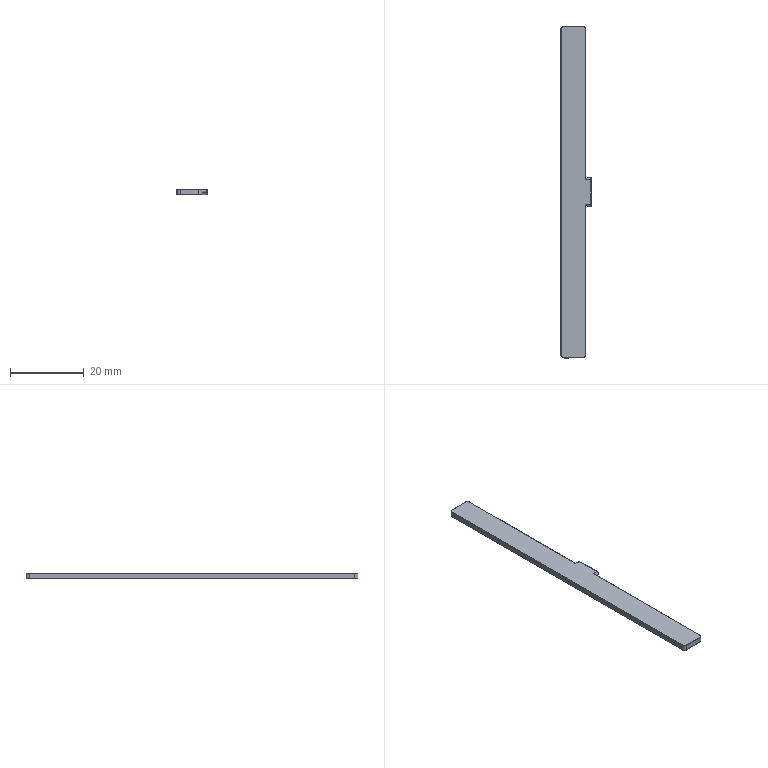Part | SolidWorks | features BaseBody 1, Fillet 1 | 1 solid | 40 faces | box 8.2 x 89.8 x 1.6 mm | volume 989.322 mm3 | cylinder 18 | torus 12 | plane 8 | spline 2 | commonest cylinder face diameters 0.2 x11 1.8 x4 1 x2 20 x1
STEP:
#1=CARTESIAN_POINT('',(-0.735,0.,12.4));
#2=VERTEX_POINT('',#1);
#3=CARTESIAN_POINT('',(-0.735,-3.498,13.032));
#4=VERTEX_POINT('',#3);
#5=CARTESIAN_POINT('',(-0.735,0.,22.4));
#6=DIRECTION('',(-1.,0.,0.));
#7=DIRECTION('',(0.,0.,-1.));
#8=AXIS2_PLACEMENT_3D('',#5,#6,#7);
#9=CIRCLE('',#8,10.);
#10=EDGE_CURVE('',#2,#4,#9,.T.);
#11=ORIENTED_EDGE('',*,*,#10,.F.);
#12=CARTESIAN_POINT('',(-0.635,0.,12.5));
#13=VERTEX_POINT('',#12);
#14=CARTESIAN_POINT('',(-0.735,0.,12.5));
#15=DIRECTION('',(0.,-1.,0.));
#16=DIRECTION('',(0.,0.,-1.));
#17=AXIS2_PLACEMENT_3D('',#14,#15,#16);
#18=CIRCLE('',#17,0.1);
#19=EDGE_CURVE('',#2,#13,#18,.T.);
#20=ORIENTED_EDGE('',*,*,#19,.T.);
#21=CARTESIAN_POINT('',(-0.635,-3.463,13.125));
#22=VERTEX_POINT('',#21);
#23=CARTESIAN_POINT('',(-0.635,0.,22.4));
#24=DIRECTION('',(1.,0.,0.));
#25=DIRECTION('',(0.,0.,-1.));
#26=AXIS2_PLACEMENT_3D('',#23,#24,#25);
#27=CIRCLE('',#26,9.9);
#28=EDGE_CURVE('',#22,#13,#27,.T.);
#29=ORIENTED_EDGE('',*,*,#28,.F.);
#30=CARTESIAN_POINT('',(-0.735,-3.463,13.125));
#31=DIRECTION('',(0.,-0.9368,0.3498));
#32=DIRECTION('',(0.,-0.3498,-0.9368));
#33=AXIS2_PLACEMENT_3D('',#30,#31,#32);
#34=CIRCLE('',#33,0.1);
#35=EDGE_CURVE('',#4,#22,#34,.T.);
#36=ORIENTED_EDGE('',*,*,#35,.F.);
#37=EDGE_LOOP('',(#11,#20,#29,#36));
#38=FACE_OUTER_BOUND('',#37,.T.);
#39=CARTESIAN_POINT('',(-0.735,0.,22.4));
#40=DIRECTION('',(1.,0.,0.));
#41=DIRECTION('',(0.,0.,-1.));
#42=AXIS2_PLACEMENT_3D('',#39,#40,#41);
#43=TOROIDAL_SURFACE('',#42,9.9,0.1);
#44=ADVANCED_FACE('',(#38),#43,.T.);
#45=CARTESIAN_POINT('',(-2.135,-3.323,14.));
#46=VERTEX_POINT('',#45);
#47=CARTESIAN_POINT('',(-0.735,-3.323,14.));
#48=VERTEX_POINT('',#47);
#49=CARTESIAN_POINT('',(-7.935,-3.323,14.));
#50=DIRECTION('',(1.,0.,0.));
#51=VECTOR('',#50,1000.);
#52=LINE('',#49,#51);
#53=EDGE_CURVE('',#46,#48,#52,.T.);
#54=ORIENTED_EDGE('',*,*,#53,.T.);
#55=CARTESIAN_POINT('',(-0.735,3.323,14.));
#56=VERTEX_POINT('',#55);
#57=CARTESIAN_POINT('',(-0.735,44.,14.));
#58=DIRECTION('',(0.,1.,0.));
#59=VECTOR('',#58,1000.);
#60=LINE('',#57,#59);
#61=EDGE_CURVE('',#48,#56,#60,.T.);
#62=ORIENTED_EDGE('',*,*,#61,.T.);
#63=CARTESIAN_POINT('',(-2.135,3.323,14.));
#64=VERTEX_POINT('',#63);
#65=CARTESIAN_POINT('',(-7.935,3.323,14.));
#66=DIRECTION('',(-1.,0.,0.));
#67=VECTOR('',#66,1000.);
#68=LINE('',#65,#67);
#69=EDGE_CURVE('',#56,#64,#68,.T.);
#70=ORIENTED_EDGE('',*,*,#69,.T.);
#71=CARTESIAN_POINT('',(-2.135,44.,14.));
#72=VERTEX_POINT('',#71);
#73=CARTESIAN_POINT('',(-2.135,44.,14.));
#74=DIRECTION('',(0.,1.,0.));
#75=VECTOR('',#74,1000.);
#76=LINE('',#73,#75);
#77=EDGE_CURVE('',#64,#72,#76,.T.);
#78=ORIENTED_EDGE('',*,*,#77,.T.);
#79=CARTESIAN_POINT('',(-2.935,44.8,14.));
#80=VERTEX_POINT('',#79);
#81=CARTESIAN_POINT('',(-2.935,44.,14.));
#82=DIRECTION('',(0.,0.,1.));
#83=DIRECTION('',(1.,0.,0.));
#84=AXIS2_PLACEMENT_3D('',#81,#82,#83);
#85=CIRCLE('',#84,0.8);
#86=EDGE_CURVE('',#72,#80,#85,.T.);
#87=ORIENTED_EDGE('',*,*,#86,.T.);
#88=CARTESIAN_POINT('',(-7.935,44.8,14.));
#89=VERTEX_POINT('',#88);
#90=CARTESIAN_POINT('',(-7.935,44.8,14.));
#91=DIRECTION('',(-1.,0.,0.));
#92=VECTOR('',#91,1000.);
#93=LINE('',#90,#92);
#94=EDGE_CURVE('',#80,#89,#93,.T.);
#95=ORIENTED_EDGE('',*,*,#94,.T.);
#96=CARTESIAN_POINT('',(-8.735,44.,14.));
#97=VERTEX_POINT('',#96);
#98=CARTESIAN_POINT('',(-7.935,44.,14.));
#99=DIRECTION('',(0.,0.,1.));
#100=DIRECTION('',(1.,0.,0.));
#101=AXIS2_PLACEMENT_3D('',#98,#99,#100);
#102=CIRCLE('',#101,0.8);
#103=EDGE_CURVE('',#89,#97,#102,.T.);
#104=ORIENTED_EDGE('',*,*,#103,.T.);
#105=CARTESIAN_POINT('',(-8.735,-44.,14.));
#106=VERTEX_POINT('',#105);
#107=CARTESIAN_POINT('',(-8.735,-44.,14.));
#108=DIRECTION('',(0.,-1.,0.));
#109=VECTOR('',#108,1000.);
#110=LINE('',#107,#109);
#111=EDGE_CURVE('',#97,#106,#110,.T.);
#112=ORIENTED_EDGE('',*,*,#111,.T.);
#113=CARTESIAN_POINT('',(-7.935,-44.8,14.));
#114=VERTEX_POINT('',#113);
#115=CARTESIAN_POINT('',(-7.935,-44.,14.));
#116=DIRECTION('',(0.,0.,1.));
#117=DIRECTION('',(1.,0.,0.));
#118=AXIS2_PLACEMENT_3D('',#115,#116,#117);
#119=CIRCLE('',#118,0.8);
#120=EDGE_CURVE('',#106,#114,#119,.T.);
#121=ORIENTED_EDGE('',*,*,#120,.T.);
#122=CARTESIAN_POINT('',(-2.935,-44.8,14.));
#123=VERTEX_POINT('',#122);
#124=CARTESIAN_POINT('',(-2.935,-44.8,14.));
#125=DIRECTION('',(1.,0.,0.));
#126=VECTOR('',#125,1000.);
#127=LINE('',#124,#126);
#128=EDGE_CURVE('',#114,#123,#127,.T.);
#129=ORIENTED_EDGE('',*,*,#128,.T.);
#130=CARTESIAN_POINT('',(-2.135,-44.,14.));
#131=VERTEX_POINT('',#130);
#132=CARTESIAN_POINT('',(-2.935,-44.,14.));
#133=DIRECTION('',(0.,0.,1.));
#134=DIRECTION('',(1.,0.,0.));
#135=AXIS2_PLACEMENT_3D('',#132,#133,#134);
#136=CIRCLE('',#135,0.8);
#137=EDGE_CURVE('',#123,#131,#136,.T.);
#138=ORIENTED_EDGE('',*,*,#137,.T.);
#139=CARTESIAN_POINT('',(-2.135,-3.323,14.));
#140=DIRECTION('',(0.,1.,0.));
#141=VECTOR('',#140,1000.);
#142=LINE('',#139,#141);
#143=EDGE_CURVE('',#131,#46,#142,.T.);
#144=ORIENTED_EDGE('',*,*,#143,.T.);
#145=EDGE_LOOP('',(#54,#62,#70,#78,#87,#95,#104,#112,#121,#129,#138,#144));
#146=FACE_OUTER_BOUND('',#145,.T.);
#147=CARTESIAN_POINT('',(-7.935,44.,14.));
#148=DIRECTION('',(0.,0.,1.));
#149=DIRECTION('',(1.,0.,0.));
#150=AXIS2_PLACEMENT_3D('',#147,#148,#149);
#151=PLANE('',#150);
#152=ADVANCED_FACE('',(#146),#151,.T.);
#153=CARTESIAN_POINT('',(-2.035,-3.498,13.032));
#154=VERTEX_POINT('',#153);
#155=CARTESIAN_POINT('',(-0.635,-3.498,13.032));
#156=DIRECTION('',(-1.,0.,0.));
#157=VECTOR('',#156,1000.);
#158=LINE('',#155,#157);
#159=EDGE_CURVE('',#4,#154,#158,.T.);
#160=ORIENTED_EDGE('',*,*,#159,.F.);
#161=CARTESIAN_POINT('',(-0.735,-3.323,13.5));
#162=DIRECTION('',(-1.,0.,0.));
#163=DIRECTION('',(0.,0.,-1.));
#164=AXIS2_PLACEMENT_3D('',#161,#162,#163);
#165=CIRCLE('',#164,0.5);
#166=EDGE_CURVE('',#4,#48,#165,.T.);
#167=ORIENTED_EDGE('',*,*,#166,.T.);
#168=ORIENTED_EDGE('',*,*,#53,.F.);
#169=CARTESIAN_POINT('',(-2.035,-3.623,13.9));
#170=VERTEX_POINT('',#169);
#171=CARTESIAN_POINT('',(-2.135,-3.323,14.));
#172=CARTESIAN_POINT('',(-2.112,-3.374,14.));
#173=CARTESIAN_POINT('',(-2.089,-3.426,13.992));
#174=CARTESIAN_POINT('',(-2.051,-3.527,13.959));
#175=CARTESIAN_POINT('',(-2.035,-3.577,13.934));
#176=CARTESIAN_POINT('',(-2.035,-3.623,13.9));
#177=B_SPLINE_CURVE_WITH_KNOTS('',3,(#171,#172,#173,#174,#175,#176),.UNSPECIFIED.,.F.,.F.,(4,2,4),(-0.000004472,0.0001655,0.0003354),.UNSPECIFIED.);
#178=EDGE_CURVE('',#46,#170,#177,.T.);
#179=ORIENTED_EDGE('',*,*,#178,.T.);
#180=CARTESIAN_POINT('',(-2.035,-3.323,13.5));
#181=DIRECTION('',(1.,0.,0.));
#182=DIRECTION('',(0.,0.,1.));
#183=AXIS2_PLACEMENT_3D('',#180,#181,#182);
#184=CIRCLE('',#183,0.5);
#185=EDGE_CURVE('',#170,#154,#184,.T.);
#186=ORIENTED_EDGE('',*,*,#185,.T.);
#187=EDGE_LOOP('',(#160,#167,#168,#179,#186));
#188=FACE_OUTER_BOUND('',#187,.T.);
#189=CARTESIAN_POINT('',(-0.635,-3.323,13.5));
#190=DIRECTION('',(-1.,0.,0.));
#191=DIRECTION('',(0.,0.,1.));
#192=AXIS2_PLACEMENT_3D('',#189,#190,#191);
#193=CYLINDRICAL_SURFACE('',#192,0.5);
#194=ADVANCED_FACE('',(#188),#193,.T.);
#195=ORIENTED_EDGE('',*,*,#185,.F.);
#196=CARTESIAN_POINT('',(-2.035,-44.,13.9));
#197=VERTEX_POINT('',#196);
#198=CARTESIAN_POINT('',(-2.035,-44.,13.9));
#199=DIRECTION('',(0.,-1.,0.));
#200=VECTOR('',#199,1000.);
#201=LINE('',#198,#200);
#202=EDGE_CURVE('',#170,#197,#201,.T.);
#203=ORIENTED_EDGE('',*,*,#202,.T.);
#204=CARTESIAN_POINT('',(-2.035,-44.,12.5));
#205=VERTEX_POINT('',#204);
#206=CARTESIAN_POINT('',(-2.035,-44.,14.));
#207=DIRECTION('',(0.,0.,1.));
#208=VECTOR('',#207,1000.);
#209=LINE('',#206,#208);
#210=EDGE_CURVE('',#205,#197,#209,.T.);
#211=ORIENTED_EDGE('',*,*,#210,.F.);
#212=CARTESIAN_POINT('',(-2.035,-1.411,12.5));
#213=VERTEX_POINT('',#212);
#214=CARTESIAN_POINT('',(-2.035,-44.,12.5));
#215=DIRECTION('',(0.,1.,0.));
#216=VECTOR('',#215,1000.);
#217=LINE('',#214,#216);
#218=EDGE_CURVE('',#205,#213,#217,.T.);
#219=ORIENTED_EDGE('',*,*,#218,.T.);
#220=CARTESIAN_POINT('',(-2.035,0.,22.4));
#221=DIRECTION('',(1.,0.,0.));
#222=DIRECTION('',(0.,0.,1.));
#223=AXIS2_PLACEMENT_3D('',#220,#221,#222);
#224=CIRCLE('',#223,10.);
#225=EDGE_CURVE('',#154,#213,#224,.T.);
#226=ORIENTED_EDGE('',*,*,#225,.F.);
#227=EDGE_LOOP('',(#195,#203,#211,#219,#226));
#228=FACE_OUTER_BOUND('',#227,.T.);
#229=CARTESIAN_POINT('',(-2.035,-44.,14.));
#230=DIRECTION('',(-1.,0.,0.));
#231=DIRECTION('',(0.,0.,1.));
#232=AXIS2_PLACEMENT_3D('',#229,#230,#231);
#233=PLANE('',#232);
#234=ADVANCED_FACE('',(#228),#233,.F.);
#235=ORIENTED_EDGE('',*,*,#210,.T.);
#236=CARTESIAN_POINT('',(-2.935,-44.9,13.9));
#237=VERTEX_POINT('',#236);
#238=CARTESIAN_POINT('',(-2.935,-44.,13.9));
#239=DIRECTION('',(0.,0.,-1.));
#240=DIRECTION('',(1.,0.,0.));
#241=AXIS2_PLACEMENT_3D('',#238,#239,#240);
#242=CIRCLE('',#241,0.9);
#243=EDGE_CURVE('',#197,#237,#242,.T.);
#244=ORIENTED_EDGE('',*,*,#243,.T.);
#245=CARTESIAN_POINT('',(-2.935,-44.9,12.5));
#246=VERTEX_POINT('',#245);
#247=CARTESIAN_POINT('',(-2.935,-44.9,14.));
#248=DIRECTION('',(0.,0.,-1.));
#249=VECTOR('',#248,1000.);
#250=LINE('',#247,#249);
#251=EDGE_CURVE('',#237,#246,#250,.T.);
#252=ORIENTED_EDGE('',*,*,#251,.T.);
#253=CARTESIAN_POINT('',(-2.935,-44.,12.5));
#254=DIRECTION('',(0.,0.,1.));
#255=DIRECTION('',(1.,0.,0.));
#256=AXIS2_PLACEMENT_3D('',#253,#254,#255);
#257=CIRCLE('',#256,0.9);
#258=EDGE_CURVE('',#246,#205,#257,.T.);
#259=ORIENTED_EDGE('',*,*,#258,.T.);
#260=EDGE_LOOP('',(#235,#244,#252,#259));
#261=FACE_OUTER_BOUND('',#260,.T.);
#262=CARTESIAN_POINT('',(-2.935,-44.,14.));
#263=DIRECTION('',(0.,0.,-1.));
#264=DIRECTION('',(-1.,0.,0.));
#265=AXIS2_PLACEMENT_3D('',#262,#263,#264);
#266=CYLINDRICAL_SURFACE('',#265,0.9);
#267=ADVANCED_FACE('',(#261),#266,.T.);
#268=ORIENTED_EDGE('',*,*,#251,.F.);
#269=CARTESIAN_POINT('',(-7.935,-44.9,13.9));
#270=VERTEX_POINT('',#269);
#271=CARTESIAN_POINT('',(-7.935,-44.9,13.9));
#272=DIRECTION('',(-1.,0.,0.));
#273=VECTOR('',#272,1000.);
#274=LINE('',#271,#273);
#275=EDGE_CURVE('',#237,#270,#274,.T.);
#276=ORIENTED_EDGE('',*,*,#275,.T.);
#277=CARTESIAN_POINT('',(-7.935,-44.9,12.5));
#278=VERTEX_POINT('',#277);
#279=CARTESIAN_POINT('',(-7.935,-44.9,14.));
#280=DIRECTION('',(0.,0.,1.));
#281=VECTOR('',#280,1000.);
#282=LINE('',#279,#281);
#283=EDGE_CURVE('',#278,#270,#282,.T.);
#284=ORIENTED_EDGE('',*,*,#283,.F.);
#285=CARTESIAN_POINT('',(-7.935,-44.9,12.5));
#286=DIRECTION('',(1.,0.,0.));
#287=VECTOR('',#286,1000.);
#288=LINE('',#285,#287);
#289=EDGE_CURVE('',#278,#246,#288,.T.);
#290=ORIENTED_EDGE('',*,*,#289,.T.);
#291=EDGE_LOOP('',(#268,#276,#284,#290));
#292=FACE_OUTER_BOUND('',#291,.T.);
#293=CARTESIAN_POINT('',(-7.935,-44.9,14.));
#294=DIRECTION('',(0.,1.,0.));
#295=DIRECTION('',(0.,0.,1.));
#296=AXIS2_PLACEMENT_3D('',#293,#294,#295);
#297=PLANE('',#296);
#298=ADVANCED_FACE('',(#292),#297,.F.);
#299=ORIENTED_EDGE('',*,*,#283,.T.);
#300=CARTESIAN_POINT('',(-8.835,-44.,13.9));
#301=VERTEX_POINT('',#300);
#302=CARTESIAN_POINT('',(-7.935,-44.,13.9));
#303=DIRECTION('',(0.,0.,-1.));
#304=DIRECTION('',(1.,0.,0.));
#305=AXIS2_PLACEMENT_3D('',#302,#303,#304);
#306=CIRCLE('',#305,0.9);
#307=EDGE_CURVE('',#270,#301,#306,.T.);
#308=ORIENTED_EDGE('',*,*,#307,.T.);
#309=CARTESIAN_POINT('',(-8.835,-44.,12.5));
#310=VERTEX_POINT('',#309);
#311=CARTESIAN_POINT('',(-8.835,-44.,14.));
#312=DIRECTION('',(0.,0.,-1.));
#313=VECTOR('',#312,1000.);
#314=LINE('',#311,#313);
#315=EDGE_CURVE('',#301,#310,#314,.T.);
#316=ORIENTED_EDGE('',*,*,#315,.T.);
#317=CARTESIAN_POINT('',(-7.935,-44.,12.5));
#318=DIRECTION('',(0.,0.,1.));
#319=DIRECTION('',(1.,0.,0.));
#320=AXIS2_PLACEMENT_3D('',#317,#318,#319);
#321=CIRCLE('',#320,0.9);
#322=EDGE_CURVE('',#310,#278,#321,.T.);
#323=ORIENTED_EDGE('',*,*,#322,.T.);
#324=EDGE_LOOP('',(#299,#308,#316,#323));
#325=FACE_OUTER_BOUND('',#324,.T.);
#326=CARTESIAN_POINT('',(-7.935,-44.,14.));
#327=DIRECTION('',(0.,0.,-1.));
#328=DIRECTION('',(-1.,0.,0.));
#329=AXIS2_PLACEMENT_3D('',#326,#327,#328);
#330=CYLINDRICAL_SURFACE('',#329,0.9);
#331=ADVANCED_FACE('',(#325),#330,.T.);
#332=ORIENTED_EDGE('',*,*,#315,.F.);
#333=CARTESIAN_POINT('',(-8.835,44.,13.9));
#334=VERTEX_POINT('',#333);
#335=CARTESIAN_POINT('',(-8.835,44.,13.9));
#336=DIRECTION('',(0.,1.,0.));
#337=VECTOR('',#336,1000.);
#338=LINE('',#335,#337);
#339=EDGE_CURVE('',#301,#334,#338,.T.);
#340=ORIENTED_EDGE('',*,*,#339,.T.);
#341=CARTESIAN_POINT('',(-8.835,44.,12.5));
#342=VERTEX_POINT('',#341);
#343=CARTESIAN_POINT('',(-8.835,44.,14.));
#344=DIRECTION('',(0.,0.,1.));
#345=VECTOR('',#344,1000.);
#346=LINE('',#343,#345);
#347=EDGE_CURVE('',#342,#334,#346,.T.);
#348=ORIENTED_EDGE('',*,*,#347,.F.);
#349=CARTESIAN_POINT('',(-8.835,44.,12.5));
#350=DIRECTION('',(0.,-1.,0.));
#351=VECTOR('',#350,1000.);
#352=LINE('',#349,#351);
#353=EDGE_CURVE('',#342,#310,#352,.T.);
#354=ORIENTED_EDGE('',*,*,#353,.T.);
#355=EDGE_LOOP('',(#332,#340,#348,#354));
#356=FACE_OUTER_BOUND('',#355,.T.);
#357=CARTESIAN_POINT('',(-8.835,44.,14.));
#358=DIRECTION('',(1.,0.,0.));
#359=DIRECTION('',(0.,0.,-1.));
#360=AXIS2_PLACEMENT_3D('',#357,#358,#359);
#361=PLANE('',#360);
#362=ADVANCED_FACE('',(#356),#361,.F.);
#363=ORIENTED_EDGE('',*,*,#347,.T.);
#364=CARTESIAN_POINT('',(-7.935,44.9,13.9));
#365=VERTEX_POINT('',#364);
#366=CARTESIAN_POINT('',(-7.935,44.,13.9));
#367=DIRECTION('',(0.,0.,-1.));
#368=DIRECTION('',(1.,0.,0.));
#369=AXIS2_PLACEMENT_3D('',#366,#367,#368);
#370=CIRCLE('',#369,0.9);
#371=EDGE_CURVE('',#334,#365,#370,.T.);
#372=ORIENTED_EDGE('',*,*,#371,.T.);
#373=CARTESIAN_POINT('',(-7.935,44.9,12.5));
#374=VERTEX_POINT('',#373);
#375=CARTESIAN_POINT('',(-7.935,44.9,14.));
#376=DIRECTION('',(0.,0.,-1.));
#377=VECTOR('',#376,1000.);
#378=LINE('',#375,#377);
#379=EDGE_CURVE('',#365,#374,#378,.T.);
#380=ORIENTED_EDGE('',*,*,#379,.T.);
#381=CARTESIAN_POINT('',(-7.935,44.,12.5));
#382=DIRECTION('',(0.,0.,1.));
#383=DIRECTION('',(1.,0.,0.));
#384=AXIS2_PLACEMENT_3D('',#381,#382,#383);
#385=CIRCLE('',#384,0.9);
#386=EDGE_CURVE('',#374,#342,#385,.T.);
#387=ORIENTED_EDGE('',*,*,#386,.T.);
#388=EDGE_LOOP('',(#363,#372,#380,#387));
#389=FACE_OUTER_BOUND('',#388,.T.);
#390=CARTESIAN_POINT('',(-7.935,44.,14.));
#391=DIRECTION('',(0.,0.,-1.));
#392=DIRECTION('',(-1.,0.,0.));
#393=AXIS2_PLACEMENT_3D('',#390,#391,#392);
#394=CYLINDRICAL_SURFACE('',#393,0.9);
#395=ADVANCED_FACE('',(#389),#394,.T.);
#396=ORIENTED_EDGE('',*,*,#379,.F.);
#397=CARTESIAN_POINT('',(-2.935,44.9,13.9));
#398=VERTEX_POINT('',#397);
#399=CARTESIAN_POINT('',(-2.935,44.9,13.9));
#400=DIRECTION('',(1.,0.,0.));
#401=VECTOR('',#400,1000.);
#402=LINE('',#399,#401);
#403=EDGE_CURVE('',#365,#398,#402,.T.);
#404=ORIENTED_EDGE('',*,*,#403,.T.);
#405=CARTESIAN_POINT('',(-2.935,44.9,12.5));
#406=VERTEX_POINT('',#405);
#407=CARTESIAN_POINT('',(-2.935,44.9,14.));
#408=DIRECTION('',(0.,0.,1.));
#409=VECTOR('',#408,1000.);
#410=LINE('',#407,#409);
#411=EDGE_CURVE('',#406,#398,#410,.T.);
#412=ORIENTED_EDGE('',*,*,#411,.F.);
#413=CARTESIAN_POINT('',(-2.935,44.9,12.5));
#414=DIRECTION('',(-1.,0.,0.));
#415=VECTOR('',#414,1000.);
#416=LINE('',#413,#415);
#417=EDGE_CURVE('',#406,#374,#416,.T.);
#418=ORIENTED_EDGE('',*,*,#417,.T.);
#419=EDGE_LOOP('',(#396,#404,#412,#418));
#420=FACE_OUTER_BOUND('',#419,.T.);
#421=CARTESIAN_POINT('',(-2.935,44.9,14.));
#422=DIRECTION('',(0.,-1.,0.));
#423=DIRECTION('',(0.,0.,-1.));
#424=AXIS2_PLACEMENT_3D('',#421,#422,#423);
#425=PLANE('',#424);
#426=ADVANCED_FACE('',(#420),#425,.F.);
#427=ORIENTED_EDGE('',*,*,#411,.T.);
#428=CARTESIAN_POINT('',(-2.035,44.,13.9));
#429=VERTEX_POINT('',#428);
#430=CARTESIAN_POINT('',(-2.935,44.,13.9));
#431=DIRECTION('',(0.,0.,-1.));
#432=DIRECTION('',(1.,0.,0.));
#433=AXIS2_PLACEMENT_3D('',#430,#431,#432);
#434=CIRCLE('',#433,0.9);
#435=EDGE_CURVE('',#398,#429,#434,.T.);
#436=ORIENTED_EDGE('',*,*,#435,.T.);
#437=CARTESIAN_POINT('',(-2.035,44.,12.5));
#438=VERTEX_POINT('',#437);
#439=CARTESIAN_POINT('',(-2.035,44.,14.));
#440=DIRECTION('',(0.,0.,-1.));
#441=VECTOR('',#440,1000.);
#442=LINE('',#439,#441);
#443=EDGE_CURVE('',#429,#438,#442,.T.);
#444=ORIENTED_EDGE('',*,*,#443,.T.);
#445=CARTESIAN_POINT('',(-2.935,44.,12.5));
#446=DIRECTION('',(0.,0.,1.));
#447=DIRECTION('',(1.,0.,0.));
#448=AXIS2_PLACEMENT_3D('',#445,#446,#447);
#449=CIRCLE('',#448,0.9);
#450=EDGE_CURVE('',#438,#406,#449,.T.);
#451=ORIENTED_EDGE('',*,*,#450,.T.);
#452=EDGE_LOOP('',(#427,#436,#444,#451));
#453=FACE_OUTER_BOUND('',#452,.T.);
#454=CARTESIAN_POINT('',(-2.935,44.,14.));
#455=DIRECTION('',(0.,0.,-1.));
#456=DIRECTION('',(-1.,0.,0.));
#457=AXIS2_PLACEMENT_3D('',#454,#455,#456);
#458=CYLINDRICAL_SURFACE('',#457,0.9);
#459=ADVANCED_FACE('',(#453),#458,.T.);
#460=ORIENTED_EDGE('',*,*,#443,.F.);
#461=CARTESIAN_POINT('',(-2.035,3.623,13.9));
#462=VERTEX_POINT('',#461);
#463=CARTESIAN_POINT('',(-2.035,3.323,13.9));
#464=DIRECTION('',(0.,-1.,0.));
#465=VECTOR('',#464,1000.);
#466=LINE('',#463,#465);
#467=EDGE_CURVE('',#429,#462,#466,.T.);
#468=ORIENTED_EDGE('',*,*,#467,.T.);
#469=CARTESIAN_POINT('',(-2.035,3.498,13.032));
#470=VERTEX_POINT('',#469);
#471=CARTESIAN_POINT('',(-2.035,3.323,13.5));
#472=DIRECTION('',(1.,0.,0.));
#473=DIRECTION('',(0.,0.,1.));
#474=AXIS2_PLACEMENT_3D('',#471,#472,#473);
#475=CIRCLE('',#474,0.5);
#476=EDGE_CURVE('',#470,#462,#475,.T.);
#477=ORIENTED_EDGE('',*,*,#476,.F.);
#478=CARTESIAN_POINT('',(-2.035,1.411,12.5));
#479=VERTEX_POINT('',#478);
#480=CARTESIAN_POINT('',(-2.035,0.,22.4));
#481=DIRECTION('',(1.,0.,0.));
#482=DIRECTION('',(0.,0.,1.));
#483=AXIS2_PLACEMENT_3D('',#480,#481,#482);
#484=CIRCLE('',#483,10.);
#485=EDGE_CURVE('',#479,#470,#484,.T.);
#486=ORIENTED_EDGE('',*,*,#485,.F.);
#487=CARTESIAN_POINT('',(-2.035,-44.,12.5));
#488=DIRECTION('',(0.,1.,0.));
#489=VECTOR('',#488,1000.);
#490=LINE('',#487,#489);
#491=EDGE_CURVE('',#479,#438,#490,.T.);
#492=ORIENTED_EDGE('',*,*,#491,.T.);
#493=EDGE_LOOP('',(#460,#468,#477,#486,#492));
#494=FACE_OUTER_BOUND('',#493,.T.);
#495=CARTESIAN_POINT('',(-2.035,-44.,14.));
#496=DIRECTION('',(-1.,0.,0.));
#497=DIRECTION('',(0.,0.,1.));
#498=AXIS2_PLACEMENT_3D('',#495,#496,#497);
#499=PLANE('',#498);
#500=ADVANCED_FACE('',(#494),#499,.F.);
#501=ORIENTED_EDGE('',*,*,#69,.F.);
#502=CARTESIAN_POINT('',(-0.735,3.498,13.032));
#503=VERTEX_POINT('',#502);
#504=CARTESIAN_POINT('',(-0.735,3.323,13.5));
#505=DIRECTION('',(-1.,0.,0.));
#506=DIRECTION('',(0.,0.,-1.));
#507=AXIS2_PLACEMENT_3D('',#504,#505,#506);
#508=CIRCLE('',#507,0.5);
#509=EDGE_CURVE('',#56,#503,#508,.T.);
#510=ORIENTED_EDGE('',*,*,#509,.T.);
#511=CARTESIAN_POINT('',(-0.635,3.498,13.032));
#512=DIRECTION('',(-1.,0.,0.));
#513=VECTOR('',#512,1000.);
#514=LINE('',#511,#513);
#515=EDGE_CURVE('',#503,#470,#514,.T.);
#516=ORIENTED_EDGE('',*,*,#515,.T.);
#517=ORIENTED_EDGE('',*,*,#476,.T.);
#518=CARTESIAN_POINT('',(-2.035,3.623,13.9));
#519=CARTESIAN_POINT('',(-2.035,3.577,13.934));
#520=CARTESIAN_POINT('',(-2.051,3.527,13.959));
#521=CARTESIAN_POINT('',(-2.089,3.426,13.992));
#522=CARTESIAN_POINT('',(-2.112,3.374,14.));
#523=CARTESIAN_POINT('',(-2.135,3.323,14.));
#524=B_SPLINE_CURVE_WITH_KNOTS('',3,(#518,#519,#520,#521,#522,#523),.UNSPECIFIED.,.F.,.F.,(4,2,4),(0.,0.0001693,0.0003386),.UNSPECIFIED.);
#525=EDGE_CURVE('',#462,#64,#524,.T.);
#526=ORIENTED_EDGE('',*,*,#525,.T.);
#527=EDGE_LOOP('',(#501,#510,#516,#517,#526));
#528=FACE_OUTER_BOUND('',#527,.T.);
#529=CARTESIAN_POINT('',(-0.635,3.323,13.5));
#530=DIRECTION('',(-1.,0.,0.));
#531=DIRECTION('',(0.,0.,1.));
#532=AXIS2_PLACEMENT_3D('',#529,#530,#531);
#533=CYLINDRICAL_SURFACE('',#532,0.5);
#534=ADVANCED_FACE('',(#528),#533,.T.);
#535=CARTESIAN_POINT('',(-0.635,3.323,13.9));
#536=VERTEX_POINT('',#535);
#537=CARTESIAN_POINT('',(-0.635,-3.323,13.9));
#538=VERTEX_POINT('',#537);
#539=CARTESIAN_POINT('',(-0.635,0.,13.9));
#540=DIRECTION('',(0.,-1.,0.));
#541=VECTOR('',#540,1000.);
#542=LINE('',#539,#541);
#543=EDGE_CURVE('',#536,#538,#542,.T.);
#544=ORIENTED_EDGE('',*,*,#543,.T.);
#545=CARTESIAN_POINT('',(-0.635,-3.323,13.5));
#546=DIRECTION('',(1.,0.,0.));
#547=DIRECTION('',(0.,0.,-1.));
#548=AXIS2_PLACEMENT_3D('',#545,#546,#547);
#549=CIRCLE('',#548,0.4);
#550=EDGE_CURVE('',#538,#22,#549,.T.);
#551=ORIENTED_EDGE('',*,*,#550,.T.);
#552=ORIENTED_EDGE('',*,*,#28,.T.);
#553=CARTESIAN_POINT('',(-0.635,3.463,13.125));
#554=VERTEX_POINT('',#553);
#555=CARTESIAN_POINT('',(-0.635,0.,22.4));
#556=DIRECTION('',(1.,0.,0.));
#557=DIRECTION('',(0.,0.,-1.));
#558=AXIS2_PLACEMENT_3D('',#555,#556,#557);
#559=CIRCLE('',#558,9.9);
#560=EDGE_CURVE('',#13,#554,#559,.T.);
#561=ORIENTED_EDGE('',*,*,#560,.T.);
#562=CARTESIAN_POINT('',(-0.635,3.323,13.5));
#563=DIRECTION('',(1.,0.,0.));
#564=DIRECTION('',(0.,0.,-1.));
#565=AXIS2_PLACEMENT_3D('',#562,#563,#564);
#566=CIRCLE('',#565,0.4);
#567=EDGE_CURVE('',#554,#536,#566,.T.);
#568=ORIENTED_EDGE('',*,*,#567,.T.);
#569=EDGE_LOOP('',(#544,#551,#552,#561,#568));
#570=FACE_OUTER_BOUND('',#569,.T.);
#571=CARTESIAN_POINT('',(-0.635,0.,22.4));
#572=DIRECTION('',(1.,0.,0.));
#573=DIRECTION('',(0.,0.,-1.));
#574=AXIS2_PLACEMENT_3D('',#571,#572,#573);
#575=PLANE('',#574);
#576=ADVANCED_FACE('',(#570),#575,.T.);
#577=ORIENTED_EDGE('',*,*,#515,.F.);
#578=CARTESIAN_POINT('',(-0.735,0.,22.4));
#579=DIRECTION('',(-1.,0.,0.));
#580=DIRECTION('',(0.,0.,-1.));
#581=AXIS2_PLACEMENT_3D('',#578,#579,#580);
#582=CIRCLE('',#581,10.);
#583=EDGE_CURVE('',#503,#2,#582,.T.);
#584=ORIENTED_EDGE('',*,*,#583,.T.);
#585=ORIENTED_EDGE('',*,*,#10,.T.);
#586=ORIENTED_EDGE('',*,*,#159,.T.);
#587=ORIENTED_EDGE('',*,*,#225,.T.);
#588=CARTESIAN_POINT('',(-2.035,0.,12.4));
#589=VERTEX_POINT('',#588);
#590=CARTESIAN_POINT('',(-2.035,0.,22.4));
#591=DIRECTION('',(1.,0.,0.));
#592=DIRECTION('',(0.,0.,1.));
#593=AXIS2_PLACEMENT_3D('',#590,#591,#592);
#594=CIRCLE('',#593,10.);
#595=EDGE_CURVE('',#213,#589,#594,.T.);
#596=ORIENTED_EDGE('',*,*,#595,.T.);
#597=CARTESIAN_POINT('',(-2.035,0.,22.4));
#598=DIRECTION('',(1.,0.,0.));
#599=DIRECTION('',(0.,0.,1.));
#600=AXIS2_PLACEMENT_3D('',#597,#598,#599);
#601=CIRCLE('',#600,10.);
#602=EDGE_CURVE('',#589,#479,#601,.T.);
#603=ORIENTED_EDGE('',*,*,#602,.T.);
#604=ORIENTED_EDGE('',*,*,#485,.T.);
#605=EDGE_LOOP('',(#577,#584,#585,#586,#587,#596,#603,#604));
#606=FACE_OUTER_BOUND('',#605,.T.);
#607=CARTESIAN_POINT('',(-0.635,0.,22.4));
#608=DIRECTION('',(-1.,0.,0.));
#609=DIRECTION('',(0.,0.,1.));
#610=AXIS2_PLACEMENT_3D('',#607,#608,#609);
#611=CYLINDRICAL_SURFACE('',#610,10.);
#612=ADVANCED_FACE('',(#606),#611,.T.);
#613=CARTESIAN_POINT('',(-2.935,-44.8,12.4));
#614=VERTEX_POINT('',#613);
#615=CARTESIAN_POINT('',(-7.935,-44.8,12.4));
#616=VERTEX_POINT('',#615);
#617=CARTESIAN_POINT('',(-7.935,-44.8,12.4));
#618=DIRECTION('',(-1.,0.,0.));
#619=VECTOR('',#618,1000.);
#620=LINE('',#617,#619);
#621=EDGE_CURVE('',#614,#616,#620,.T.);
#622=ORIENTED_EDGE('',*,*,#621,.T.);
#623=CARTESIAN_POINT('',(-8.735,-44.,12.4));
#624=VERTEX_POINT('',#623);
#625=CARTESIAN_POINT('',(-7.935,-44.,12.4));
#626=DIRECTION('',(0.,0.,-1.));
#627=DIRECTION('',(1.,0.,0.));
#628=AXIS2_PLACEMENT_3D('',#625,#626,#627);
#629=CIRCLE('',#628,0.8);
#630=EDGE_CURVE('',#616,#624,#629,.T.);
#631=ORIENTED_EDGE('',*,*,#630,.T.);
#632=CARTESIAN_POINT('',(-8.735,44.,12.4));
#633=VERTEX_POINT('',#632);
#634=CARTESIAN_POINT('',(-8.735,44.,12.4));
#635=DIRECTION('',(0.,1.,0.));
#636=VECTOR('',#635,1000.);
#637=LINE('',#634,#636);
#638=EDGE_CURVE('',#624,#633,#637,.T.);
#639=ORIENTED_EDGE('',*,*,#638,.T.);
#640=CARTESIAN_POINT('',(-7.935,44.8,12.4));
#641=VERTEX_POINT('',#640);
#642=CARTESIAN_POINT('',(-7.935,44.,12.4));
#643=DIRECTION('',(0.,0.,-1.));
#644=DIRECTION('',(1.,0.,0.));
#645=AXIS2_PLACEMENT_3D('',#642,#643,#644);
#646=CIRCLE('',#645,0.8);
#647=EDGE_CURVE('',#633,#641,#646,.T.);
#648=ORIENTED_EDGE('',*,*,#647,.T.);
#649=CARTESIAN_POINT('',(-2.935,44.8,12.4));
#650=VERTEX_POINT('',#649);
#651=CARTESIAN_POINT('',(-7.935,44.8,12.4));
#652=DIRECTION('',(1.,0.,0.));
#653=VECTOR('',#652,1000.);
#654=LINE('',#651,#653);
#655=EDGE_CURVE('',#641,#650,#654,.T.);
#656=ORIENTED_EDGE('',*,*,#655,.T.);
#657=CARTESIAN_POINT('',(-2.135,44.,12.4));
#658=VERTEX_POINT('',#657);
#659=CARTESIAN_POINT('',(-2.935,44.,12.4));
#660=DIRECTION('',(0.,0.,-1.));
#661=DIRECTION('',(1.,0.,0.));
#662=AXIS2_PLACEMENT_3D('',#659,#660,#661);
#663=CIRCLE('',#662,0.8);
#664=EDGE_CURVE('',#650,#658,#663,.T.);
#665=ORIENTED_EDGE('',*,*,#664,.T.);
#666=CARTESIAN_POINT('',(-2.135,1.411,12.4));
#667=VERTEX_POINT('',#666);
#668=CARTESIAN_POINT('',(-2.135,44.,12.4));
#669=DIRECTION('',(0.,-1.,0.));
#670=VECTOR('',#669,1000.);
#671=LINE('',#668,#670);
#672=EDGE_CURVE('',#658,#667,#671,.T.);
#673=ORIENTED_EDGE('',*,*,#672,.T.);
#674=CARTESIAN_POINT('',(-2.135,1.411,12.4));
#675=CARTESIAN_POINT('',(-2.135,1.175,12.4));
#676=CARTESIAN_POINT('',(-2.12,0.9394,12.4));
#677=CARTESIAN_POINT('',(-2.082,0.4693,12.4));
#678=CARTESIAN_POINT('',(-2.059,0.2345,12.4));
#679=CARTESIAN_POINT('',(-2.035,0.,12.4));
#680=B_SPLINE_CURVE_WITH_KNOTS('',3,(#674,#675,#676,#677,#678,#679),.UNSPECIFIED.,.F.,.F.,(4,2,4),(0.,0.0007072,0.001414),.UNSPECIFIED.);
#681=EDGE_CURVE('',#667,#589,#680,.T.);
#682=ORIENTED_EDGE('',*,*,#681,.T.);
#683=CARTESIAN_POINT('',(-2.135,-1.411,12.4));
#684=VERTEX_POINT('',#683);
#685=CARTESIAN_POINT('',(-2.035,0.,12.4));
#686=CARTESIAN_POINT('',(-2.059,-0.2346,12.4));
#687=CARTESIAN_POINT('',(-2.082,-0.4693,12.4));
#688=CARTESIAN_POINT('',(-2.12,-0.9394,12.4));
#689=CARTESIAN_POINT('',(-2.135,-1.175,12.4));
#690=CARTESIAN_POINT('',(-2.135,-1.411,12.4));
#691=B_SPLINE_CURVE_WITH_KNOTS('',3,(#685,#686,#687,#688,#689,#690),.UNSPECIFIED.,.F.,.F.,(4,2,4),(-0.0000199,0.0006875,0.001395),.UNSPECIFIED.);
#692=EDGE_CURVE('',#589,#684,#691,.T.);
#693=ORIENTED_EDGE('',*,*,#692,.T.);
#694=CARTESIAN_POINT('',(-2.135,-44.,12.4));
#695=VERTEX_POINT('',#694);
#696=CARTESIAN_POINT('',(-2.135,44.,12.4));
#697=DIRECTION('',(0.,-1.,0.));
#698=VECTOR('',#697,1000.);
#699=LINE('',#696,#698);
#700=EDGE_CURVE('',#684,#695,#699,.T.);
#701=ORIENTED_EDGE('',*,*,#700,.T.);
#702=CARTESIAN_POINT('',(-2.935,-44.,12.4));
#703=DIRECTION('',(0.,0.,-1.));
#704=DIRECTION('',(1.,0.,0.));
#705=AXIS2_PLACEMENT_3D('',#702,#703,#704);
#706=CIRCLE('',#705,0.8);
#707=EDGE_CURVE('',#695,#614,#706,.T.);
#708=ORIENTED_EDGE('',*,*,#707,.T.);
#709=EDGE_LOOP('',(#622,#631,#639,#648,#656,#665,#673,#682,#693,#701,#708));
#710=FACE_OUTER_BOUND('',#709,.T.);
#711=CARTESIAN_POINT('',(-7.935,44.,12.4));
#712=DIRECTION('',(0.,0.,1.));
#713=DIRECTION('',(1.,0.,0.));
#714=AXIS2_PLACEMENT_3D('',#711,#712,#713);
#715=PLANE('',#714);
#716=ADVANCED_FACE('',(#710),#715,.F.);
#717=CARTESIAN_POINT('',(-0.735,3.323,13.9));
#718=DIRECTION('',(0.,-1.,0.));
#719=DIRECTION('',(0.,0.,-1.));
#720=AXIS2_PLACEMENT_3D('',#717,#718,#719);
#721=CIRCLE('',#720,0.1);
#722=EDGE_CURVE('',#536,#56,#721,.T.);
#723=ORIENTED_EDGE('',*,*,#722,.F.);
#724=ORIENTED_EDGE('',*,*,#567,.F.);
#725=CARTESIAN_POINT('',(-0.735,3.463,13.125));
#726=DIRECTION('',(0.,-0.9368,-0.3498));
#727=DIRECTION('',(0.,0.3498,-0.9368));
#728=AXIS2_PLACEMENT_3D('',#725,#726,#727);
#729=CIRCLE('',#728,0.1);
#730=EDGE_CURVE('',#503,#554,#729,.T.);
#731=ORIENTED_EDGE('',*,*,#730,.F.);
#732=ORIENTED_EDGE('',*,*,#509,.F.);
#733=EDGE_LOOP('',(#723,#724,#731,#732));
#734=FACE_OUTER_BOUND('',#733,.T.);
#735=CARTESIAN_POINT('',(-0.735,3.323,13.5));
#736=DIRECTION('',(1.,0.,0.));
#737=DIRECTION('',(0.,0.,-1.));
#738=AXIS2_PLACEMENT_3D('',#735,#736,#737);
#739=TOROIDAL_SURFACE('',#738,0.4,0.1);
#740=ADVANCED_FACE('',(#734),#739,.T.);
#741=ORIENTED_EDGE('',*,*,#19,.F.);
#742=ORIENTED_EDGE('',*,*,#583,.F.);
#743=ORIENTED_EDGE('',*,*,#730,.T.);
#744=ORIENTED_EDGE('',*,*,#560,.F.);
#745=EDGE_LOOP('',(#741,#742,#743,#744));
#746=FACE_OUTER_BOUND('',#745,.T.);
#747=CARTESIAN_POINT('',(-0.735,0.,22.4));
#748=DIRECTION('',(1.,0.,0.));
#749=DIRECTION('',(0.,0.,-1.));
#750=AXIS2_PLACEMENT_3D('',#747,#748,#749);
#751=TOROIDAL_SURFACE('',#750,9.9,0.1);
#752=ADVANCED_FACE('',(#746),#751,.T.);
#753=ORIENTED_EDGE('',*,*,#722,.T.);
#754=ORIENTED_EDGE('',*,*,#61,.F.);
#755=CARTESIAN_POINT('',(-0.735,-3.323,13.9));
#756=DIRECTION('',(0.,-1.,0.));
#757=DIRECTION('',(0.,0.,-1.));
#758=AXIS2_PLACEMENT_3D('',#755,#756,#757);
#759=CIRCLE('',#758,0.1);
#760=EDGE_CURVE('',#538,#48,#759,.T.);
#761=ORIENTED_EDGE('',*,*,#760,.F.);
#762=ORIENTED_EDGE('',*,*,#543,.F.);
#763=EDGE_LOOP('',(#753,#754,#761,#762));
#764=FACE_OUTER_BOUND('',#763,.T.);
#765=CARTESIAN_POINT('',(-0.735,44.,13.9));
#766=DIRECTION('',(0.,1.,0.));
#767=DIRECTION('',(0.,0.,1.));
#768=AXIS2_PLACEMENT_3D('',#765,#766,#767);
#769=CYLINDRICAL_SURFACE('',#768,0.1);
#770=ADVANCED_FACE('',(#764),#769,.T.);
#771=ORIENTED_EDGE('',*,*,#35,.T.);
#772=ORIENTED_EDGE('',*,*,#550,.F.);
#773=ORIENTED_EDGE('',*,*,#760,.T.);
#774=ORIENTED_EDGE('',*,*,#166,.F.);
#775=EDGE_LOOP('',(#771,#772,#773,#774));
#776=FACE_OUTER_BOUND('',#775,.T.);
#777=CARTESIAN_POINT('',(-0.735,-3.323,13.5));
#778=DIRECTION('',(1.,0.,0.));
#779=DIRECTION('',(0.,0.,-1.));
#780=AXIS2_PLACEMENT_3D('',#777,#778,#779);
#781=TOROIDAL_SURFACE('',#780,0.4,0.1);
#782=ADVANCED_FACE('',(#776),#781,.T.);
#783=ORIENTED_EDGE('',*,*,#525,.F.);
#784=ORIENTED_EDGE('',*,*,#467,.F.);
#785=CARTESIAN_POINT('',(-2.135,44.,13.9));
#786=DIRECTION('',(0.,1.,0.));
#787=DIRECTION('',(0.,0.,1.));
#788=AXIS2_PLACEMENT_3D('',#785,#786,#787);
#789=CIRCLE('',#788,0.1);
#790=EDGE_CURVE('',#72,#429,#789,.T.);
#791=ORIENTED_EDGE('',*,*,#790,.F.);
#792=ORIENTED_EDGE('',*,*,#77,.F.);
#793=EDGE_LOOP('',(#783,#784,#791,#792));
#794=FACE_OUTER_BOUND('',#793,.T.);
#795=CARTESIAN_POINT('',(-2.135,44.,13.9));
#796=DIRECTION('',(0.,-1.,0.));
#797=DIRECTION('',(0.,0.,-1.));
#798=AXIS2_PLACEMENT_3D('',#795,#796,#797);
#799=CYLINDRICAL_SURFACE('',#798,0.1);
#800=ADVANCED_FACE('',(#794),#799,.T.);
#801=ORIENTED_EDGE('',*,*,#790,.T.);
#802=ORIENTED_EDGE('',*,*,#435,.F.);
#803=CARTESIAN_POINT('',(-2.935,44.8,13.9));
#804=DIRECTION('',(-1.,0.,0.));
#805=DIRECTION('',(0.,0.,1.));
#806=AXIS2_PLACEMENT_3D('',#803,#804,#805);
#807=CIRCLE('',#806,0.1);
#808=EDGE_CURVE('',#80,#398,#807,.T.);
#809=ORIENTED_EDGE('',*,*,#808,.F.);
#810=ORIENTED_EDGE('',*,*,#86,.F.);
#811=EDGE_LOOP('',(#801,#802,#809,#810));
#812=FACE_OUTER_BOUND('',#811,.T.);
#813=CARTESIAN_POINT('',(-2.935,44.,13.9));
#814=DIRECTION('',(0.,0.,1.));
#815=DIRECTION('',(1.,0.,0.));
#816=AXIS2_PLACEMENT_3D('',#813,#814,#815);
#817=TOROIDAL_SURFACE('',#816,0.8,0.1);
#818=ADVANCED_FACE('',(#812),#817,.T.);
#819=ORIENTED_EDGE('',*,*,#808,.T.);
#820=ORIENTED_EDGE('',*,*,#403,.F.);
#821=CARTESIAN_POINT('',(-7.935,44.8,13.9));
#822=DIRECTION('',(-1.,0.,0.));
#823=DIRECTION('',(0.,0.,1.));
#824=AXIS2_PLACEMENT_3D('',#821,#822,#823);
#825=CIRCLE('',#824,0.1);
#826=EDGE_CURVE('',#89,#365,#825,.T.);
#827=ORIENTED_EDGE('',*,*,#826,.F.);
#828=ORIENTED_EDGE('',*,*,#94,.F.);
#829=EDGE_LOOP('',(#819,#820,#827,#828));
#830=FACE_OUTER_BOUND('',#829,.T.);
#831=CARTESIAN_POINT('',(-7.935,44.8,13.9));
#832=DIRECTION('',(1.,0.,0.));
#833=DIRECTION('',(0.,0.,-1.));
#834=AXIS2_PLACEMENT_3D('',#831,#832,#833);
#835=CYLINDRICAL_SURFACE('',#834,0.1);
#836=ADVANCED_FACE('',(#830),#835,.T.);
#837=ORIENTED_EDGE('',*,*,#826,.T.);
#838=ORIENTED_EDGE('',*,*,#371,.F.);
#839=CARTESIAN_POINT('',(-8.735,44.,13.9));
#840=DIRECTION('',(0.,-1.,0.));
#841=DIRECTION('',(0.,0.,-1.));
#842=AXIS2_PLACEMENT_3D('',#839,#840,#841);
#843=CIRCLE('',#842,0.1);
#844=EDGE_CURVE('',#97,#334,#843,.T.);
#845=ORIENTED_EDGE('',*,*,#844,.F.);
#846=ORIENTED_EDGE('',*,*,#103,.F.);
#847=EDGE_LOOP('',(#837,#838,#845,#846));
#848=FACE_OUTER_BOUND('',#847,.T.);
#849=CARTESIAN_POINT('',(-7.935,44.,13.9));
#850=DIRECTION('',(0.,0.,1.));
#851=DIRECTION('',(1.,0.,0.));
#852=AXIS2_PLACEMENT_3D('',#849,#850,#851);
#853=TOROIDAL_SURFACE('',#852,0.8,0.1);
#854=ADVANCED_FACE('',(#848),#853,.T.);
#855=ORIENTED_EDGE('',*,*,#844,.T.);
#856=ORIENTED_EDGE('',*,*,#339,.F.);
#857=CARTESIAN_POINT('',(-8.735,-44.,13.9));
#858=DIRECTION('',(0.,-1.,0.));
#859=DIRECTION('',(0.,0.,-1.));
#860=AXIS2_PLACEMENT_3D('',#857,#858,#859);
#861=CIRCLE('',#860,0.1);
#862=EDGE_CURVE('',#106,#301,#861,.T.);
#863=ORIENTED_EDGE('',*,*,#862,.F.);
#864=ORIENTED_EDGE('',*,*,#111,.F.);
#865=EDGE_LOOP('',(#855,#856,#863,#864));
#866=FACE_OUTER_BOUND('',#865,.T.);
#867=CARTESIAN_POINT('',(-8.735,44.,13.9));
#868=DIRECTION('',(0.,1.,0.));
#869=DIRECTION('',(0.,0.,1.));
#870=AXIS2_PLACEMENT_3D('',#867,#868,#869);
#871=CYLINDRICAL_SURFACE('',#870,0.1);
#872=ADVANCED_FACE('',(#866),#871,.T.);
#873=ORIENTED_EDGE('',*,*,#862,.T.);
#874=ORIENTED_EDGE('',*,*,#307,.F.);
#875=CARTESIAN_POINT('',(-7.935,-44.8,13.9));
#876=DIRECTION('',(1.,0.,0.));
#877=DIRECTION('',(0.,0.,-1.));
#878=AXIS2_PLACEMENT_3D('',#875,#876,#877);
#879=CIRCLE('',#878,0.1);
#880=EDGE_CURVE('',#114,#270,#879,.T.);
#881=ORIENTED_EDGE('',*,*,#880,.F.);
#882=ORIENTED_EDGE('',*,*,#120,.F.);
#883=EDGE_LOOP('',(#873,#874,#881,#882));
#884=FACE_OUTER_BOUND('',#883,.T.);
#885=CARTESIAN_POINT('',(-7.935,-44.,13.9));
#886=DIRECTION('',(0.,0.,1.));
#887=DIRECTION('',(1.,0.,0.));
#888=AXIS2_PLACEMENT_3D('',#885,#886,#887);
#889=TOROIDAL_SURFACE('',#888,0.8,0.1);
#890=ADVANCED_FACE('',(#884),#889,.T.);
#891=ORIENTED_EDGE('',*,*,#880,.T.);
#892=ORIENTED_EDGE('',*,*,#275,.F.);
#893=CARTESIAN_POINT('',(-2.935,-44.8,13.9));
#894=DIRECTION('',(1.,0.,0.));
#895=DIRECTION('',(0.,0.,-1.));
#896=AXIS2_PLACEMENT_3D('',#893,#894,#895);
#897=CIRCLE('',#896,0.1);
#898=EDGE_CURVE('',#123,#237,#897,.T.);
#899=ORIENTED_EDGE('',*,*,#898,.F.);
#900=ORIENTED_EDGE('',*,*,#128,.F.);
#901=EDGE_LOOP('',(#891,#892,#899,#900));
#902=FACE_OUTER_BOUND('',#901,.T.);
#903=CARTESIAN_POINT('',(-7.935,-44.8,13.9));
#904=DIRECTION('',(-1.,0.,0.));
#905=DIRECTION('',(0.,0.,1.));
#906=AXIS2_PLACEMENT_3D('',#903,#904,#905);
#907=CYLINDRICAL_SURFACE('',#906,0.1);
#908=ADVANCED_FACE('',(#902),#907,.T.);
#909=ORIENTED_EDGE('',*,*,#178,.F.);
#910=ORIENTED_EDGE('',*,*,#143,.F.);
#911=CARTESIAN_POINT('',(-2.135,-44.,13.9));
#912=DIRECTION('',(0.,-1.,0.));
#913=DIRECTION('',(0.,0.,-1.));
#914=AXIS2_PLACEMENT_3D('',#911,#912,#913);
#915=CIRCLE('',#914,0.1);
#916=EDGE_CURVE('',#197,#131,#915,.T.);
#917=ORIENTED_EDGE('',*,*,#916,.F.);
#918=ORIENTED_EDGE('',*,*,#202,.F.);
#919=EDGE_LOOP('',(#909,#910,#917,#918));
#920=FACE_OUTER_BOUND('',#919,.T.);
#921=CARTESIAN_POINT('',(-2.135,44.,13.9));
#922=DIRECTION('',(0.,-1.,0.));
#923=DIRECTION('',(0.,0.,-1.));
#924=AXIS2_PLACEMENT_3D('',#921,#922,#923);
#925=CYLINDRICAL_SURFACE('',#924,0.1);
#926=ADVANCED_FACE('',(#920),#925,.T.);
#927=ORIENTED_EDGE('',*,*,#898,.T.);
#928=ORIENTED_EDGE('',*,*,#243,.F.);
#929=ORIENTED_EDGE('',*,*,#916,.T.);
#930=ORIENTED_EDGE('',*,*,#137,.F.);
#931=EDGE_LOOP('',(#927,#928,#929,#930));
#932=FACE_OUTER_BOUND('',#931,.T.);
#933=CARTESIAN_POINT('',(-2.935,-44.,13.9));
#934=DIRECTION('',(0.,0.,1.));
#935=DIRECTION('',(1.,0.,0.));
#936=AXIS2_PLACEMENT_3D('',#933,#934,#935);
#937=TOROIDAL_SURFACE('',#936,0.8,0.1);
#938=ADVANCED_FACE('',(#932),#937,.T.);
#939=ORIENTED_EDGE('',*,*,#692,.F.);
#940=ORIENTED_EDGE('',*,*,#595,.F.);
#941=CARTESIAN_POINT('',(-2.135,-1.411,12.5));
#942=DIRECTION('',(0.,-1.,0.));
#943=DIRECTION('',(1.,0.,0.));
#944=AXIS2_PLACEMENT_3D('',#941,#942,#943);
#945=CIRCLE('',#944,0.1);
#946=EDGE_CURVE('',#684,#213,#945,.T.);
#947=ORIENTED_EDGE('',*,*,#946,.F.);
#948=EDGE_LOOP('',(#939,#940,#947));
#949=FACE_OUTER_BOUND('',#948,.T.);
#950=CARTESIAN_POINT('',(-2.135,-1.411,12.4));
#951=CARTESIAN_POINT('',(-2.035,-1.411,12.4));
#952=CARTESIAN_POINT('',(-2.035,-1.411,12.5));
#953=CARTESIAN_POINT('',(-2.135,-1.175,12.4));
#954=CARTESIAN_POINT('',(-2.063,-1.212,12.4));
#955=CARTESIAN_POINT('',(-2.035,-1.18,12.467));
#956=CARTESIAN_POINT('',(-2.12,-0.9399,12.4));
#957=CARTESIAN_POINT('',(-2.068,-0.9554,12.4));
#958=CARTESIAN_POINT('',(-2.035,-0.9458,12.442));
#959=CARTESIAN_POINT('',(-2.082,-0.4697,12.4));
#960=CARTESIAN_POINT('',(-2.059,-0.4829,12.4));
#961=CARTESIAN_POINT('',(-2.035,-0.4744,12.408));
#962=CARTESIAN_POINT('',(-2.059,-0.2353,12.4));
#963=CARTESIAN_POINT('',(-2.047,-0.2365,12.4));
#964=CARTESIAN_POINT('',(-2.035,-0.2377,12.4));
#965=CARTESIAN_POINT('',(-2.035,0.,12.4));
#966=CARTESIAN_POINT('',(-2.035,0.,12.4));
#967=CARTESIAN_POINT('',(-2.035,0.,12.4));
#968=(BOUNDED_SURFACE()B_SPLINE_SURFACE(3,2,((#950,#951,#952),(#953,#954,#955),(#956,#957,#958),(#959,#960,#961),(#962,#963,#964),(#965,#966,#967)),.UNSPECIFIED.,.F.,.F.,.T.)B_SPLINE_SURFACE_WITH_KNOTS((4,2,4),(3,3),(0.0006234,0.001344,0.002065),(0.,1.),.UNSPECIFIED.)GEOMETRIC_REPRESENTATION_ITEM()RATIONAL_B_SPLINE_SURFACE(((1.,0.7071,1.),(1.,0.8216,1.),(1.,0.8899,1.),(1.,0.9796,1.),(1.,0.9997,1.),(1.,1.,1.)))REPRESENTATION_ITEM('')SURFACE());
#969=ADVANCED_FACE('',(#949),#968,.T.);
#970=ORIENTED_EDGE('',*,*,#946,.T.);
#971=ORIENTED_EDGE('',*,*,#218,.F.);
#972=CARTESIAN_POINT('',(-2.135,-44.,12.5));
#973=DIRECTION('',(0.,-1.,0.));
#974=DIRECTION('',(0.,0.,-1.));
#975=AXIS2_PLACEMENT_3D('',#972,#973,#974);
#976=CIRCLE('',#975,0.1);
#977=EDGE_CURVE('',#695,#205,#976,.T.);
#978=ORIENTED_EDGE('',*,*,#977,.F.);
#979=ORIENTED_EDGE('',*,*,#700,.F.);
#980=EDGE_LOOP('',(#970,#971,#978,#979));
#981=FACE_OUTER_BOUND('',#980,.T.);
#982=CARTESIAN_POINT('',(-2.135,44.,12.5));
#983=DIRECTION('',(0.,-1.,0.));
#984=DIRECTION('',(0.,0.,-1.));
#985=AXIS2_PLACEMENT_3D('',#982,#983,#984);
#986=CYLINDRICAL_SURFACE('',#985,0.1);
#987=ADVANCED_FACE('',(#981),#986,.T.);
#988=ORIENTED_EDGE('',*,*,#602,.F.);
#989=ORIENTED_EDGE('',*,*,#681,.F.);
#990=CARTESIAN_POINT('',(-2.135,1.411,12.5));
#991=DIRECTION('',(0.,1.,0.));
#992=DIRECTION('',(-1.,0.,0.));
#993=AXIS2_PLACEMENT_3D('',#990,#991,#992);
#994=CIRCLE('',#993,0.1);
#995=EDGE_CURVE('',#479,#667,#994,.T.);
#996=ORIENTED_EDGE('',*,*,#995,.F.);
#997=EDGE_LOOP('',(#988,#989,#996));
#998=FACE_OUTER_BOUND('',#997,.T.);
#999=CARTESIAN_POINT('',(-2.035,1.411,12.5));
#1000=CARTESIAN_POINT('',(-2.035,1.411,12.4));
#1001=CARTESIAN_POINT('',(-2.135,1.411,12.4));
#1002=CARTESIAN_POINT('',(-2.035,1.18,12.467));
#1003=CARTESIAN_POINT('',(-2.063,1.212,12.4));
#1004=CARTESIAN_POINT('',(-2.135,1.175,12.4));
#1005=CARTESIAN_POINT('',(-2.035,0.9458,12.442));
#1006=CARTESIAN_POINT('',(-2.068,0.9554,12.4));
#1007=CARTESIAN_POINT('',(-2.12,0.9399,12.4));
#1008=CARTESIAN_POINT('',(-2.035,0.4744,12.408));
#1009=CARTESIAN_POINT('',(-2.059,0.4829,12.4));
#1010=CARTESIAN_POINT('',(-2.082,0.4697,12.4));
#1011=CARTESIAN_POINT('',(-2.035,0.2377,12.4));
#1012=CARTESIAN_POINT('',(-2.047,0.2365,12.4));
#1013=CARTESIAN_POINT('',(-2.059,0.2353,12.4));
#1014=CARTESIAN_POINT('',(-2.035,0.,12.4));
#1015=CARTESIAN_POINT('',(-2.035,0.,12.4));
#1016=CARTESIAN_POINT('',(-2.035,0.,12.4));
#1017=(BOUNDED_SURFACE()B_SPLINE_SURFACE(3,2,((#999,#1000,#1001),(#1002,#1003,#1004),(#1005,#1006,#1007),(#1008,#1009,#1010),(#1011,#1012,#1013),(#1014,#1015,#1016)),.UNSPECIFIED.,.F.,.F.,.T.)B_SPLINE_SURFACE_WITH_KNOTS((4,2,4),(3,3),(0.0006234,0.001344,0.002065),(0.,1.),.UNSPECIFIED.)GEOMETRIC_REPRESENTATION_ITEM()RATIONAL_B_SPLINE_SURFACE(((1.,0.7071,1.),(1.,0.8216,1.),(1.,0.8899,1.),(1.,0.9796,1.),(1.,0.9997,1.),(1.,1.,1.)))REPRESENTATION_ITEM('')SURFACE());
#1018=ADVANCED_FACE('',(#998),#1017,.T.);
#1019=ORIENTED_EDGE('',*,*,#977,.T.);
#1020=ORIENTED_EDGE('',*,*,#258,.F.);
#1021=CARTESIAN_POINT('',(-2.935,-44.8,12.5));
#1022=DIRECTION('',(-1.,0.,0.));
#1023=DIRECTION('',(0.,0.,1.));
#1024=AXIS2_PLACEMENT_3D('',#1021,#1022,#1023);
#1025=CIRCLE('',#1024,0.1);
#1026=EDGE_CURVE('',#614,#246,#1025,.T.);
#1027=ORIENTED_EDGE('',*,*,#1026,.F.);
#1028=ORIENTED_EDGE('',*,*,#707,.F.);
#1029=EDGE_LOOP('',(#1019,#1020,#1027,#1028));
#1030=FACE_OUTER_BOUND('',#1029,.T.);
#1031=CARTESIAN_POINT('',(-2.935,-44.,12.5));
#1032=DIRECTION('',(0.,0.,1.));
#1033=DIRECTION('',(1.,0.,0.));
#1034=AXIS2_PLACEMENT_3D('',#1031,#1032,#1033);
#1035=TOROIDAL_SURFACE('',#1034,0.8,0.1);
#1036=ADVANCED_FACE('',(#1030),#1035,.T.);
#1037=ORIENTED_EDGE('',*,*,#995,.T.);
#1038=ORIENTED_EDGE('',*,*,#672,.F.);
#1039=CARTESIAN_POINT('',(-2.135,44.,12.5));
#1040=DIRECTION('',(0.,1.,0.));
#1041=DIRECTION('',(0.,0.,1.));
#1042=AXIS2_PLACEMENT_3D('',#1039,#1040,#1041);
#1043=CIRCLE('',#1042,0.1);
#1044=EDGE_CURVE('',#438,#658,#1043,.T.);
#1045=ORIENTED_EDGE('',*,*,#1044,.F.);
#1046=ORIENTED_EDGE('',*,*,#491,.F.);
#1047=EDGE_LOOP('',(#1037,#1038,#1045,#1046));
#1048=FACE_OUTER_BOUND('',#1047,.T.);
#1049=CARTESIAN_POINT('',(-2.135,44.,12.5));
#1050=DIRECTION('',(0.,-1.,0.));
#1051=DIRECTION('',(0.,0.,-1.));
#1052=AXIS2_PLACEMENT_3D('',#1049,#1050,#1051);
#1053=CYLINDRICAL_SURFACE('',#1052,0.1);
#1054=ADVANCED_FACE('',(#1048),#1053,.T.);
#1055=ORIENTED_EDGE('',*,*,#1026,.T.);
#1056=ORIENTED_EDGE('',*,*,#289,.F.);
#1057=CARTESIAN_POINT('',(-7.935,-44.8,12.5));
#1058=DIRECTION('',(-1.,0.,0.));
#1059=DIRECTION('',(0.,0.,1.));
#1060=AXIS2_PLACEMENT_3D('',#1057,#1058,#1059);
#1061=CIRCLE('',#1060,0.1);
#1062=EDGE_CURVE('',#616,#278,#1061,.T.);
#1063=ORIENTED_EDGE('',*,*,#1062,.F.);
#1064=ORIENTED_EDGE('',*,*,#621,.F.);
#1065=EDGE_LOOP('',(#1055,#1056,#1063,#1064));
#1066=FACE_OUTER_BOUND('',#1065,.T.);
#1067=CARTESIAN_POINT('',(-7.935,-44.8,12.5));
#1068=DIRECTION('',(-1.,0.,0.));
#1069=DIRECTION('',(0.,0.,1.));
#1070=AXIS2_PLACEMENT_3D('',#1067,#1068,#1069);
#1071=CYLINDRICAL_SURFACE('',#1070,0.1);
#1072=ADVANCED_FACE('',(#1066),#1071,.T.);
#1073=ORIENTED_EDGE('',*,*,#1044,.T.);
#1074=ORIENTED_EDGE('',*,*,#664,.F.);
#1075=CARTESIAN_POINT('',(-2.935,44.8,12.5));
#1076=DIRECTION('',(-1.,0.,0.));
#1077=DIRECTION('',(0.,0.,1.));
#1078=AXIS2_PLACEMENT_3D('',#1075,#1076,#1077);
#1079=CIRCLE('',#1078,0.1);
#1080=EDGE_CURVE('',#406,#650,#1079,.T.);
#1081=ORIENTED_EDGE('',*,*,#1080,.F.);
#1082=ORIENTED_EDGE('',*,*,#450,.F.);
#1083=EDGE_LOOP('',(#1073,#1074,#1081,#1082));
#1084=FACE_OUTER_BOUND('',#1083,.T.);
#1085=CARTESIAN_POINT('',(-2.935,44.,12.5));
#1086=DIRECTION('',(0.,0.,1.));
#1087=DIRECTION('',(1.,0.,0.));
#1088=AXIS2_PLACEMENT_3D('',#1085,#1086,#1087);
#1089=TOROIDAL_SURFACE('',#1088,0.8,0.1);
#1090=ADVANCED_FACE('',(#1084),#1089,.T.);
#1091=ORIENTED_EDGE('',*,*,#1062,.T.);
#1092=ORIENTED_EDGE('',*,*,#322,.F.);
#1093=CARTESIAN_POINT('',(-8.735,-44.,12.5));
#1094=DIRECTION('',(0.,1.,0.));
#1095=DIRECTION('',(0.,0.,1.));
#1096=AXIS2_PLACEMENT_3D('',#1093,#1094,#1095);
#1097=CIRCLE('',#1096,0.1);
#1098=EDGE_CURVE('',#624,#310,#1097,.T.);
#1099=ORIENTED_EDGE('',*,*,#1098,.F.);
#1100=ORIENTED_EDGE('',*,*,#630,.F.);
#1101=EDGE_LOOP('',(#1091,#1092,#1099,#1100));
#1102=FACE_OUTER_BOUND('',#1101,.T.);
#1103=CARTESIAN_POINT('',(-7.935,-44.,12.5));
#1104=DIRECTION('',(0.,0.,1.));
#1105=DIRECTION('',(1.,0.,0.));
#1106=AXIS2_PLACEMENT_3D('',#1103,#1104,#1105);
#1107=TOROIDAL_SURFACE('',#1106,0.8,0.1);
#1108=ADVANCED_FACE('',(#1102),#1107,.T.);
#1109=ORIENTED_EDGE('',*,*,#1080,.T.);
#1110=ORIENTED_EDGE('',*,*,#655,.F.);
#1111=CARTESIAN_POINT('',(-7.935,44.8,12.5));
#1112=DIRECTION('',(-1.,0.,0.));
#1113=DIRECTION('',(0.,0.,1.));
#1114=AXIS2_PLACEMENT_3D('',#1111,#1112,#1113);
#1115=CIRCLE('',#1114,0.1);
#1116=EDGE_CURVE('',#374,#641,#1115,.T.);
#1117=ORIENTED_EDGE('',*,*,#1116,.F.);
#1118=ORIENTED_EDGE('',*,*,#417,.F.);
#1119=EDGE_LOOP('',(#1109,#1110,#1117,#1118));
#1120=FACE_OUTER_BOUND('',#1119,.T.);
#1121=CARTESIAN_POINT('',(-7.935,44.8,12.5));
#1122=DIRECTION('',(1.,0.,0.));
#1123=DIRECTION('',(0.,0.,-1.));
#1124=AXIS2_PLACEMENT_3D('',#1121,#1122,#1123);
#1125=CYLINDRICAL_SURFACE('',#1124,0.1);
#1126=ADVANCED_FACE('',(#1120),#1125,.T.);
#1127=ORIENTED_EDGE('',*,*,#1098,.T.);
#1128=ORIENTED_EDGE('',*,*,#353,.F.);
#1129=CARTESIAN_POINT('',(-8.735,44.,12.5));
#1130=DIRECTION('',(0.,1.,0.));
#1131=DIRECTION('',(0.,0.,1.));
#1132=AXIS2_PLACEMENT_3D('',#1129,#1130,#1131);
#1133=CIRCLE('',#1132,0.1);
#1134=EDGE_CURVE('',#633,#342,#1133,.T.);
#1135=ORIENTED_EDGE('',*,*,#1134,.F.);
#1136=ORIENTED_EDGE('',*,*,#638,.F.);
#1137=EDGE_LOOP('',(#1127,#1128,#1135,#1136));
#1138=FACE_OUTER_BOUND('',#1137,.T.);
#1139=CARTESIAN_POINT('',(-8.735,44.,12.5));
#1140=DIRECTION('',(0.,1.,0.));
#1141=DIRECTION('',(0.,0.,1.));
#1142=AXIS2_PLACEMENT_3D('',#1139,#1140,#1141);
#1143=CYLINDRICAL_SURFACE('',#1142,0.1);
#1144=ADVANCED_FACE('',(#1138),#1143,.T.);
#1145=ORIENTED_EDGE('',*,*,#1116,.T.);
#1146=ORIENTED_EDGE('',*,*,#647,.F.);
#1147=ORIENTED_EDGE('',*,*,#1134,.T.);
#1148=ORIENTED_EDGE('',*,*,#386,.F.);
#1149=EDGE_LOOP('',(#1145,#1146,#1147,#1148));
#1150=FACE_OUTER_BOUND('',#1149,.T.);
#1151=CARTESIAN_POINT('',(-7.935,44.,12.5));
#1152=DIRECTION('',(0.,0.,1.));
#1153=DIRECTION('',(1.,0.,0.));
#1154=AXIS2_PLACEMENT_3D('',#1151,#1152,#1153);
#1155=TOROIDAL_SURFACE('',#1154,0.8,0.1);
#1156=ADVANCED_FACE('',(#1150),#1155,.T.);
#1157=CLOSED_SHELL('',(#44,#152,#194,#234,#267,#298,#331,#362,#395,#426,#459,#500,#534,#576,#612,#716,#740,#752,#770,#782,#800,#818,#836,#854,#872,#890,#908,#926,#938,#969,#987,#1018,#1036,#1054,#1072,#1090,#1108,#1126,#1144,#1156));
#1158=MANIFOLD_SOLID_BREP('',#1157);
#1159=CARTESIAN_POINT('',(0.,0.,0.));
#1160=DIRECTION('',(0.,0.,1.));
#1161=DIRECTION('',(1.,0.,0.));
#1162=AXIS2_PLACEMENT_3D('',#1159,#1160,#1161);
#1163=(LENGTH_UNIT()NAMED_UNIT(*)SI_UNIT(.MILLI.,.METRE.));
#1164=UNCERTAINTY_MEASURE_WITH_UNIT(LENGTH_MEASURE(0.00001),#1163,'','');
#1165=(NAMED_UNIT(*)PLANE_ANGLE_UNIT()SI_UNIT($,.RADIAN.));
#1166=(NAMED_UNIT(*)SI_UNIT($,.STERADIAN.)SOLID_ANGLE_UNIT());
#1167=(GEOMETRIC_REPRESENTATION_CONTEXT(3)GLOBAL_UNCERTAINTY_ASSIGNED_CONTEXT((#1164))GLOBAL_UNIT_ASSIGNED_CONTEXT((#1163,#1165,#1166))REPRESENTATION_CONTEXT('',''));
#1168=ADVANCED_BREP_SHAPE_REPRESENTATION('',(#1158,#1162),#1167);